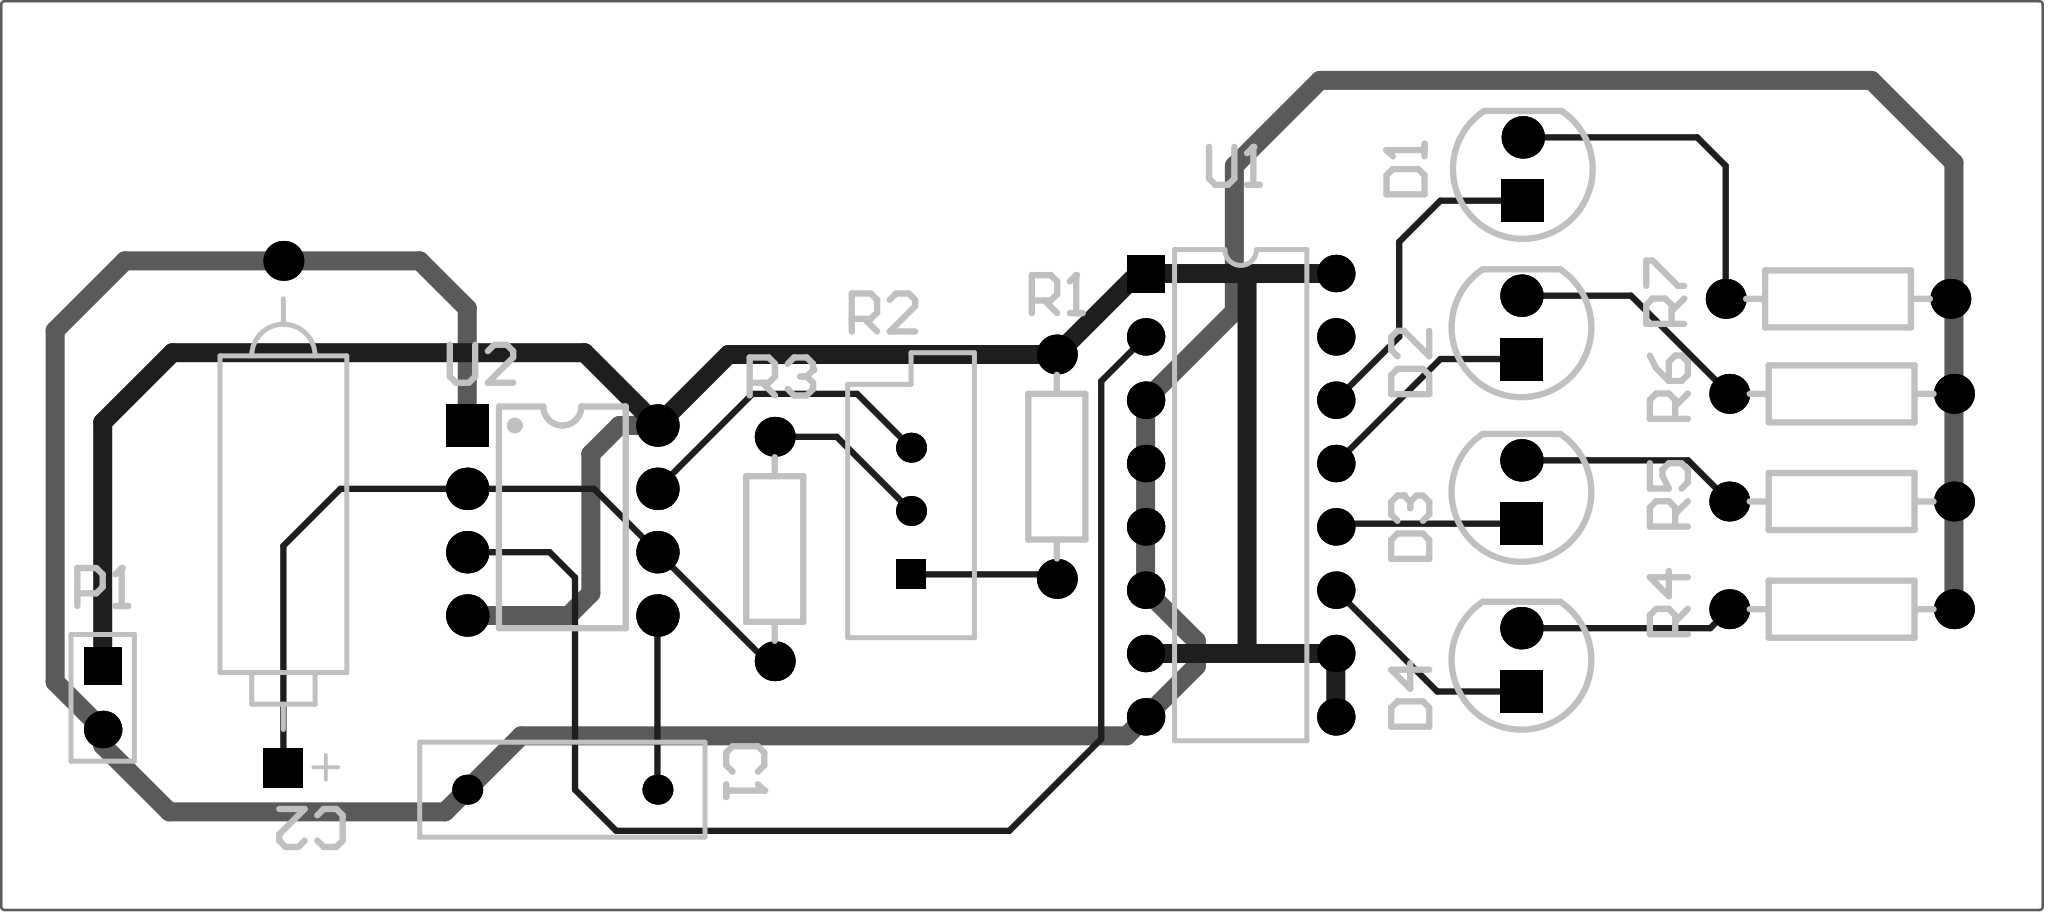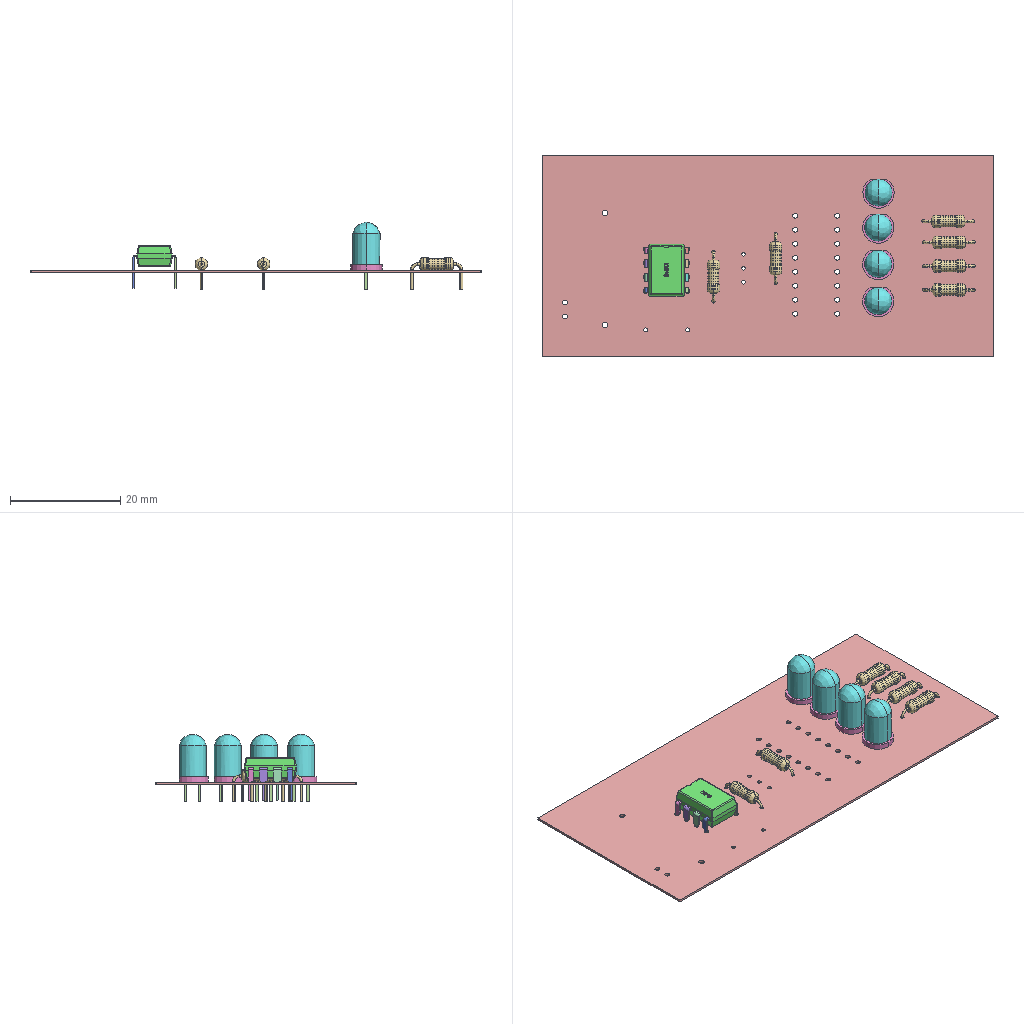Circuit board layout | Altium Designer | box 81.8 x 36.4 x 12.2 mm
Layer stack:
# Altium Designer layer stack of  (unit mm; dielectric type: 0 none, 1 core, 2 prepreg, 3 surface material)
index,name,kind,layer,copper_thickness_mm,dielectric_type,dielectric_thickness_mm,dielectric_material,dielectric_constant
0,Top Paste,other,,,,,,
1,Top Overlay,other,,,,,,
2,Top Solder,dielectric,,,3,0.0102,Solder Resist,3.5
3,Top Layer,copper,Top Layer,0.0356,,,,
4,Dielectric 1,dielectric,,,0,0.32,FR-4,4.8
5,Bottom Layer,copper,Bottom Layer,0.0356,,,,
6,Bottom Solder,dielectric,,,3,0.0102,Solder Resist,3.5
7,Bottom Overlay,other,,,,,,
8,Bottom Paste,other,,,,,,
# drill layer pairs: low layer,high layer
drill_pair,Top Layer,Bottom Layer
Part placement:
Designator,Comment,Layer,Footprint,Center-X(mm),Center-Y(mm),Rotation
C1,0.01U,TopLayer,RAD-0.3,81.153,47.879,360
C2,33U,TopLayer,POLAR0.8,69.977,58.928,270
D1,LED,TopLayer,LED_5MM-W,119.634,72.771,90
D2,LED,TopLayer,LED_5MM-W,119.579,66.421,90
D3,LED,TopLayer,LED_5MM-W,119.579,59.817,90
D4,LED,TopLayer,LED_5MM-W,119.579,53.086,90
P1,Header 2,TopLayer,HDR1X2,62.738,51.562,270
R1,10K,TopLayer,RS_1/4W,100.965,60.833,90
R2,20K,TopLayer,VR5,95.123,59.055,90
R3,10K,TopLayer,RS_1/4W,89.662,57.531,90
R4,470,TopLayer,RS_1/4W,132.406,55.118,180
R5,470,TopLayer,RS_1/4W,132.406,59.436,180
R6,470,TopLayer,RS_1/4W,132.406,63.754,180
R7,470,TopLayer,RS_1/4W,132.262,67.564,180
U1,SN74LS160AN,TopLayer,648-08,108.331,59.69,270
U2,NE555D,TopLayer,DIP8,81.153,58.674,0
Pad and via stacks:
# Altium Designer via and pad stacks of  (unit mm). Each distinct definition once, with the count of objects using it.
# via: kind,start_layer,end_layer,hole_mm,diameter_mm,mode(0 simple;1 top-mid-bottom;2 full stack),diameter_per_layer,count,example_net
# pad: kind,layer,hole_mm,hole_type(0 round;1 square;2 slot),plating,top_size,top_shape(1 round;2 rect;3 octagon;9 rounded rect),mid_size,bottom_size,mode,footprint,size_per_layer,count,example
pad,Multi-Layer,1,0,plated,1.6x1.6,2,1.6x1.6,1.6x1.6,0,POLAR0.8,,1,C2.1
pad,Multi-Layer,1,0,plated,1.6x1.6,1,1.6x1.6,1.6x1.6,0,POLAR0.8,,1,C2.2
pad,Multi-Layer,0.7,0,plated,1.2x1.2,1,1.2x1.2,1.2x1.2,0,RAD-0.3,,2,C1.1
pad,Multi-Layer,0.6,0,plated,1.6x1.6,1,1.6x1.6,1.6x1.6,0,RS 1/4W,,12,R4.1
pad,Multi-Layer,0.9,0,plated,1.7x1.7,2,1.7x1.7,1.7x1.7,0,LED 5MM-W,,4,D4.1
pad,Multi-Layer,0.9,0,plated,1.7x1.7,1,1.7x1.7,1.7x1.7,0,LED 5MM-W,,4,D4.2
pad,Multi-Layer,0.7,0,plated,1.2x1.2,1,1.2x1.2,1.2x1.2,0,VR5,,2,R2.3
pad,Multi-Layer,0.7,0,plated,1.2x1.2,2,1.2x1.2,1.2x1.2,0,VR5,,1,R2.1
pad,Multi-Layer,0.8,0,plated,1.7x1.7,2,1.7x1.7,1.7x1.7,0,DIP8,,1,U2.1
pad,Multi-Layer,0.8,0,plated,1.7x1.7,1,1.7x1.7,1.7x1.7,0,DIP8,,7,U2.2
pad,Multi-Layer,0.9,0,plated,1.5x1.5,2,1.5x1.5,1.5x1.5,0,648-08,,1,U1.1
pad,Multi-Layer,0.9,0,plated,1.5x1.5,1,1.5x1.5,1.5x1.5,0,648-08,,15,U1.2
pad,Multi-Layer,0.9,0,plated,1.5x1.5,1,1.5x1.5,1.5x1.5,0,HDR1X2,,1,P1.2
pad,Multi-Layer,0.9,0,plated,1.5x1.5,2,1.5x1.5,1.5x1.5,0,HDR1X2,,1,P1.1
Design rules, without the lines most boards share:
# Altium Designer design rules of  (exported by Altium Designer, unit mm)
# columns: name | kind | enabled | priority | scope1 | scope2 | descriptor | typed fields (field=value)
Clearance | 0 | enabled | 1 | All | All | Clearance Constraint (Gap=10mil) (All),(All) | gap=0.254
PlaneConnect | 6 | enabled | 1 | All | All | Power Plane Connect Rule(Relief Connect )(Expansion=20mil) (Conductor Width=10mil) (Air Gap=10mil) (Entries=4) (All) | relief_conductor_width=0.254 relief_entries=4 relief_expansion=0.508
PolygonConnect | 20 | enabled | 1 | All | All | Polygon Connect Rule(Relief Connect )(Conductor Width=10mil) (Relief Angle=90 Angle) (Entries=4) (Air Gap Width=10mil) (All),(All) | connect_style(0=relief,1=direct,2=none)=0 relief_conductor_width=0.254 relief_entries=4
Width | 2 | enabled | 1 | All | All | Width Constraint (Min=10mil) (Max=30mil) (Preferred=10mil) (All) |
RoutingVias | 11 | enabled | 1 | All | All | Routing Via (MinHoleWidth=28mil) (MaxHoleWidth=28mil) (PreferredHoleWidth=28mil) (MinWidth=50mil) (MaxWidth=50mil) (PreferedWidth=50mil) (All) | via_min_hole=0.7112 via_max_hole=0.7112 via_preferred_diameter=1.27 via_preferred_hole=0.7112
PasteMaskExpansion | 14 | enabled | 1 | All | All | Paste Mask Expansion (Expansion =0mil) (All) | expansion=0
SolderMaskExpansion | 13 | enabled | 1 | All | All | Solder Mask Expansion (Expansion =4mil) (All) | expansion=0.1016
DiffPairsRouting | 51 | enabled | 1 | All | All | Differential Pairs Uncoupled Length using the Gap Constraints (Min=10mil) (Max=10mil) (Prefered=10mil)  and Width Constraints (Min=15mil) (Max=15mil) (Prefered=15mil) (All) |
HoleToHoleClearance | 52 | enabled | 1 | All | All | Hole To Hole Clearance (Gap=10mil) (All),(All) | gap=0.254
MinimumSolderMaskSliver | 53 | enabled | 1 | All | All | Minimum Solder Mask Sliver (Gap=0mil) (All),(All) |
SilkToSolderMaskClearance | 54 | enabled | 1 | IsPad | All | Silk To Solder Mask (Clearance=0mil) (IsPad),(All) |
SilkToSilkClearance | 55 | enabled | 1 | All | All | Silk to Silk (Clearance=0mil) (All),(All) |
Classes set for this board:
# Altium Designer classes of  (member kind: 0 net, 1 component, 2 from-to, 3 pad, 4 layer, 5 differential pair, 6 design channel, 7 polygon, 8 structure, 9 xSignal)
# columns: class name | member kind | superclass | members
sample | 1 | no | C1; C2; D1; D2; D3; D4; P1; R1; R2; R3; R4; R5; R6; R7; U1; U2;